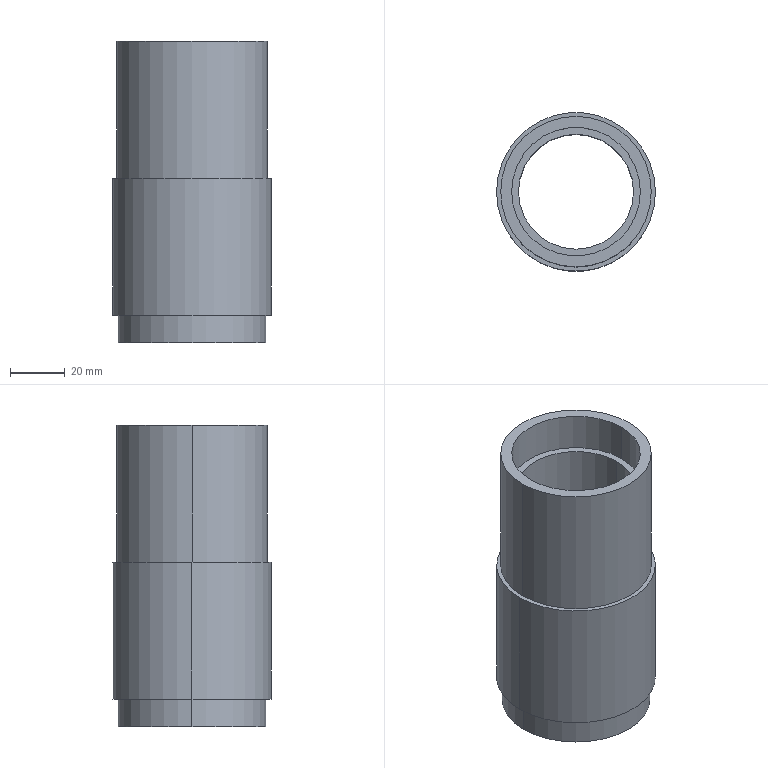Part | SolidWorks | features BaseBody 1 | 1 solid | 18 faces | box 58 x 58 x 110 mm | volume 111613 mm3 | cylinder 12 | plane 6 | commonest cylinder face diameters 47 x4 42 x2 54 x2 55 x2 58 x2
STEP:
#1=CARTESIAN_POINT('',(-27.5,0.,60.));
#2=VERTEX_POINT('',#1);
#3=CARTESIAN_POINT('',(-27.5,0.,110.));
#4=VERTEX_POINT('',#3);
#5=CARTESIAN_POINT('',(-27.5,0.,60.));
#6=DIRECTION('',(0.,0.,1.));
#7=VECTOR('',#6,1000.);
#8=LINE('',#5,#7);
#9=EDGE_CURVE('',#2,#4,#8,.T.);
#10=ORIENTED_EDGE('',*,*,#9,.F.);
#11=CARTESIAN_POINT('',(27.5,0.,60.));
#12=VERTEX_POINT('',#11);
#13=CARTESIAN_POINT('',(0.,0.,60.));
#14=DIRECTION('',(0.,0.,1.));
#15=DIRECTION('',(1.,0.,0.));
#16=AXIS2_PLACEMENT_3D('',#13,#14,#15);
#17=CIRCLE('',#16,27.5);
#18=EDGE_CURVE('',#2,#12,#17,.T.);
#19=ORIENTED_EDGE('',*,*,#18,.T.);
#20=CARTESIAN_POINT('',(27.5,0.,110.));
#21=VERTEX_POINT('',#20);
#22=CARTESIAN_POINT('',(27.5,0.,60.));
#23=DIRECTION('',(0.,0.,1.));
#24=VECTOR('',#23,1000.);
#25=LINE('',#22,#24);
#26=EDGE_CURVE('',#12,#21,#25,.T.);
#27=ORIENTED_EDGE('',*,*,#26,.T.);
#28=CARTESIAN_POINT('',(0.,0.,110.));
#29=DIRECTION('',(0.,0.,1.));
#30=DIRECTION('',(1.,0.,0.));
#31=AXIS2_PLACEMENT_3D('',#28,#29,#30);
#32=CIRCLE('',#31,27.5);
#33=EDGE_CURVE('',#4,#21,#32,.T.);
#34=ORIENTED_EDGE('',*,*,#33,.F.);
#35=EDGE_LOOP('',(#10,#19,#27,#34));
#36=FACE_OUTER_BOUND('',#35,.T.);
#37=CARTESIAN_POINT('',(0.,0.,60.));
#38=DIRECTION('',(0.,0.,1.));
#39=DIRECTION('',(1.,0.,0.));
#40=AXIS2_PLACEMENT_3D('',#37,#38,#39);
#41=CYLINDRICAL_SURFACE('',#40,27.5);
#42=ADVANCED_FACE('',(#36),#41,.T.);
#43=CARTESIAN_POINT('',(0.,0.,60.));
#44=DIRECTION('',(0.,0.,1.));
#45=DIRECTION('',(1.,0.,0.));
#46=AXIS2_PLACEMENT_3D('',#43,#44,#45);
#47=CIRCLE('',#46,27.5);
#48=EDGE_CURVE('',#12,#2,#47,.T.);
#49=ORIENTED_EDGE('',*,*,#48,.F.);
#50=ORIENTED_EDGE('',*,*,#18,.F.);
#51=EDGE_LOOP('',(#49,#50));
#52=FACE_BOUND('',#51,.T.);
#53=CARTESIAN_POINT('',(-29.,0.,60.));
#54=VERTEX_POINT('',#53);
#55=CARTESIAN_POINT('',(29.,0.,60.));
#56=VERTEX_POINT('',#55);
#57=CARTESIAN_POINT('',(0.,0.,60.));
#58=DIRECTION('',(0.,0.,1.));
#59=DIRECTION('',(1.,0.,0.));
#60=AXIS2_PLACEMENT_3D('',#57,#58,#59);
#61=CIRCLE('',#60,29.);
#62=EDGE_CURVE('',#54,#56,#61,.T.);
#63=ORIENTED_EDGE('',*,*,#62,.T.);
#64=CARTESIAN_POINT('',(0.,0.,60.));
#65=DIRECTION('',(0.,0.,1.));
#66=DIRECTION('',(1.,0.,0.));
#67=AXIS2_PLACEMENT_3D('',#64,#65,#66);
#68=CIRCLE('',#67,29.);
#69=EDGE_CURVE('',#56,#54,#68,.T.);
#70=ORIENTED_EDGE('',*,*,#69,.T.);
#71=EDGE_LOOP('',(#63,#70));
#72=FACE_OUTER_BOUND('',#71,.T.);
#73=CARTESIAN_POINT('',(0.,0.,60.));
#74=DIRECTION('',(0.,0.,1.));
#75=DIRECTION('',(1.,0.,0.));
#76=AXIS2_PLACEMENT_3D('',#73,#74,#75);
#77=PLANE('',#76);
#78=ADVANCED_FACE('',(#52,#72),#77,.T.);
#79=CARTESIAN_POINT('',(27.,0.,10.));
#80=VERTEX_POINT('',#79);
#81=CARTESIAN_POINT('',(27.,0.,0.));
#82=VERTEX_POINT('',#81);
#83=CARTESIAN_POINT('',(27.,0.,10.));
#84=DIRECTION('',(0.,0.,-1.));
#85=VECTOR('',#84,1000.);
#86=LINE('',#83,#85);
#87=EDGE_CURVE('',#80,#82,#86,.T.);
#88=ORIENTED_EDGE('',*,*,#87,.F.);
#89=CARTESIAN_POINT('',(-27.,0.,10.));
#90=VERTEX_POINT('',#89);
#91=CARTESIAN_POINT('',(0.,0.,10.));
#92=DIRECTION('',(0.,0.,-1.));
#93=DIRECTION('',(-1.,0.,0.));
#94=AXIS2_PLACEMENT_3D('',#91,#92,#93);
#95=CIRCLE('',#94,27.);
#96=EDGE_CURVE('',#80,#90,#95,.T.);
#97=ORIENTED_EDGE('',*,*,#96,.T.);
#98=CARTESIAN_POINT('',(-27.,0.,0.));
#99=VERTEX_POINT('',#98);
#100=CARTESIAN_POINT('',(-27.,0.,10.));
#101=DIRECTION('',(0.,0.,-1.));
#102=VECTOR('',#101,1000.);
#103=LINE('',#100,#102);
#104=EDGE_CURVE('',#90,#99,#103,.T.);
#105=ORIENTED_EDGE('',*,*,#104,.T.);
#106=CARTESIAN_POINT('',(0.,0.,0.));
#107=DIRECTION('',(0.,0.,-1.));
#108=DIRECTION('',(-1.,0.,0.));
#109=AXIS2_PLACEMENT_3D('',#106,#107,#108);
#110=CIRCLE('',#109,27.);
#111=EDGE_CURVE('',#82,#99,#110,.T.);
#112=ORIENTED_EDGE('',*,*,#111,.F.);
#113=EDGE_LOOP('',(#88,#97,#105,#112));
#114=FACE_OUTER_BOUND('',#113,.T.);
#115=CARTESIAN_POINT('',(0.,0.,10.));
#116=DIRECTION('',(0.,0.,-1.));
#117=DIRECTION('',(-1.,0.,0.));
#118=AXIS2_PLACEMENT_3D('',#115,#116,#117);
#119=CYLINDRICAL_SURFACE('',#118,27.);
#120=ADVANCED_FACE('',(#114),#119,.T.);
#121=CARTESIAN_POINT('',(0.,0.,10.));
#122=DIRECTION('',(0.,0.,-1.));
#123=DIRECTION('',(-1.,0.,0.));
#124=AXIS2_PLACEMENT_3D('',#121,#122,#123);
#125=CIRCLE('',#124,27.);
#126=EDGE_CURVE('',#90,#80,#125,.T.);
#127=ORIENTED_EDGE('',*,*,#126,.F.);
#128=ORIENTED_EDGE('',*,*,#96,.F.);
#129=EDGE_LOOP('',(#127,#128));
#130=FACE_BOUND('',#129,.T.);
#131=CARTESIAN_POINT('',(-29.,0.,10.));
#132=VERTEX_POINT('',#131);
#133=CARTESIAN_POINT('',(29.,0.,10.));
#134=VERTEX_POINT('',#133);
#135=CARTESIAN_POINT('',(0.,0.,10.));
#136=DIRECTION('',(0.,0.,-1.));
#137=DIRECTION('',(-1.,0.,0.));
#138=AXIS2_PLACEMENT_3D('',#135,#136,#137);
#139=CIRCLE('',#138,29.);
#140=EDGE_CURVE('',#132,#134,#139,.T.);
#141=ORIENTED_EDGE('',*,*,#140,.T.);
#142=CARTESIAN_POINT('',(0.,0.,10.));
#143=DIRECTION('',(0.,0.,-1.));
#144=DIRECTION('',(-1.,0.,0.));
#145=AXIS2_PLACEMENT_3D('',#142,#143,#144);
#146=CIRCLE('',#145,29.);
#147=EDGE_CURVE('',#134,#132,#146,.T.);
#148=ORIENTED_EDGE('',*,*,#147,.T.);
#149=EDGE_LOOP('',(#141,#148));
#150=FACE_OUTER_BOUND('',#149,.T.);
#151=CARTESIAN_POINT('',(0.,0.,10.));
#152=DIRECTION('',(0.,0.,-1.));
#153=DIRECTION('',(0.,-1.,0.));
#154=AXIS2_PLACEMENT_3D('',#151,#152,#153);
#155=PLANE('',#154);
#156=ADVANCED_FACE('',(#130,#150),#155,.T.);
#157=CARTESIAN_POINT('',(-23.5,0.,96.));
#158=VERTEX_POINT('',#157);
#159=CARTESIAN_POINT('',(-23.5,0.,110.));
#160=VERTEX_POINT('',#159);
#161=CARTESIAN_POINT('',(-23.5,0.,56.));
#162=DIRECTION('',(0.,0.,1.));
#163=VECTOR('',#162,1000.);
#164=LINE('',#161,#163);
#165=EDGE_CURVE('',#158,#160,#164,.T.);
#166=ORIENTED_EDGE('',*,*,#165,.F.);
#167=CARTESIAN_POINT('',(23.5,0.,96.));
#168=VERTEX_POINT('',#167);
#169=CARTESIAN_POINT('',(0.,0.,96.));
#170=DIRECTION('',(0.,0.,1.));
#171=DIRECTION('',(1.,0.,0.));
#172=AXIS2_PLACEMENT_3D('',#169,#170,#171);
#173=CIRCLE('',#172,23.5);
#174=EDGE_CURVE('',#168,#158,#173,.T.);
#175=ORIENTED_EDGE('',*,*,#174,.F.);
#176=CARTESIAN_POINT('',(23.5,0.,110.));
#177=VERTEX_POINT('',#176);
#178=CARTESIAN_POINT('',(23.5,0.,56.));
#179=DIRECTION('',(0.,0.,1.));
#180=VECTOR('',#179,1000.);
#181=LINE('',#178,#180);
#182=EDGE_CURVE('',#168,#177,#181,.T.);
#183=ORIENTED_EDGE('',*,*,#182,.T.);
#184=CARTESIAN_POINT('',(0.,0.,110.));
#185=DIRECTION('',(0.,0.,1.));
#186=DIRECTION('',(1.,0.,0.));
#187=AXIS2_PLACEMENT_3D('',#184,#185,#186);
#188=CIRCLE('',#187,23.5);
#189=EDGE_CURVE('',#177,#160,#188,.T.);
#190=ORIENTED_EDGE('',*,*,#189,.T.);
#191=EDGE_LOOP('',(#166,#175,#183,#190));
#192=FACE_OUTER_BOUND('',#191,.T.);
#193=CARTESIAN_POINT('',(0.,0.,56.));
#194=DIRECTION('',(0.,0.,1.));
#195=DIRECTION('',(1.,0.,0.));
#196=AXIS2_PLACEMENT_3D('',#193,#194,#195);
#197=CYLINDRICAL_SURFACE('',#196,23.5);
#198=ADVANCED_FACE('',(#192),#197,.F.);
#199=CARTESIAN_POINT('',(21.,0.,96.));
#200=VERTEX_POINT('',#199);
#201=CARTESIAN_POINT('',(-21.,0.,96.));
#202=VERTEX_POINT('',#201);
#203=CARTESIAN_POINT('',(0.,0.,96.));
#204=DIRECTION('',(0.,0.,-1.));
#205=DIRECTION('',(1.,0.,0.));
#206=AXIS2_PLACEMENT_3D('',#203,#204,#205);
#207=CIRCLE('',#206,21.);
#208=EDGE_CURVE('',#200,#202,#207,.T.);
#209=ORIENTED_EDGE('',*,*,#208,.T.);
#210=CARTESIAN_POINT('',(0.,0.,96.));
#211=DIRECTION('',(0.,0.,-1.));
#212=DIRECTION('',(1.,0.,0.));
#213=AXIS2_PLACEMENT_3D('',#210,#211,#212);
#214=CIRCLE('',#213,21.);
#215=EDGE_CURVE('',#202,#200,#214,.T.);
#216=ORIENTED_EDGE('',*,*,#215,.T.);
#217=EDGE_LOOP('',(#209,#216));
#218=FACE_BOUND('',#217,.T.);
#219=ORIENTED_EDGE('',*,*,#174,.T.);
#220=CARTESIAN_POINT('',(0.,0.,96.));
#221=DIRECTION('',(0.,0.,1.));
#222=DIRECTION('',(1.,0.,0.));
#223=AXIS2_PLACEMENT_3D('',#220,#221,#222);
#224=CIRCLE('',#223,23.5);
#225=EDGE_CURVE('',#158,#168,#224,.T.);
#226=ORIENTED_EDGE('',*,*,#225,.T.);
#227=EDGE_LOOP('',(#219,#226));
#228=FACE_OUTER_BOUND('',#227,.T.);
#229=CARTESIAN_POINT('',(0.,0.,96.));
#230=DIRECTION('',(0.,0.,1.));
#231=DIRECTION('',(1.,0.,0.));
#232=AXIS2_PLACEMENT_3D('',#229,#230,#231);
#233=PLANE('',#232);
#234=ADVANCED_FACE('',(#218,#228),#233,.T.);
#235=CARTESIAN_POINT('',(21.,0.,14.));
#236=VERTEX_POINT('',#235);
#237=CARTESIAN_POINT('',(-21.,0.,14.));
#238=VERTEX_POINT('',#237);
#239=CARTESIAN_POINT('',(0.,0.,14.));
#240=DIRECTION('',(0.,0.,-1.));
#241=DIRECTION('',(-1.,0.,0.));
#242=AXIS2_PLACEMENT_3D('',#239,#240,#241);
#243=CIRCLE('',#242,21.);
#244=EDGE_CURVE('',#236,#238,#243,.T.);
#245=ORIENTED_EDGE('',*,*,#244,.F.);
#246=CARTESIAN_POINT('',(0.,0.,14.));
#247=DIRECTION('',(0.,0.,-1.));
#248=DIRECTION('',(-1.,0.,0.));
#249=AXIS2_PLACEMENT_3D('',#246,#247,#248);
#250=CIRCLE('',#249,21.);
#251=EDGE_CURVE('',#238,#236,#250,.T.);
#252=ORIENTED_EDGE('',*,*,#251,.F.);
#253=EDGE_LOOP('',(#245,#252));
#254=FACE_BOUND('',#253,.T.);
#255=CARTESIAN_POINT('',(-23.5,0.,14.));
#256=VERTEX_POINT('',#255);
#257=CARTESIAN_POINT('',(23.5,0.,14.));
#258=VERTEX_POINT('',#257);
#259=CARTESIAN_POINT('',(0.,0.,14.));
#260=DIRECTION('',(0.,0.,-1.));
#261=DIRECTION('',(-1.,0.,0.));
#262=AXIS2_PLACEMENT_3D('',#259,#260,#261);
#263=CIRCLE('',#262,23.5);
#264=EDGE_CURVE('',#256,#258,#263,.T.);
#265=ORIENTED_EDGE('',*,*,#264,.T.);
#266=CARTESIAN_POINT('',(0.,0.,14.));
#267=DIRECTION('',(0.,0.,-1.));
#268=DIRECTION('',(-1.,0.,0.));
#269=AXIS2_PLACEMENT_3D('',#266,#267,#268);
#270=CIRCLE('',#269,23.5);
#271=EDGE_CURVE('',#258,#256,#270,.T.);
#272=ORIENTED_EDGE('',*,*,#271,.T.);
#273=EDGE_LOOP('',(#265,#272));
#274=FACE_OUTER_BOUND('',#273,.T.);
#275=CARTESIAN_POINT('',(0.,0.,14.));
#276=DIRECTION('',(0.,0.,-1.));
#277=DIRECTION('',(0.,-1.,0.));
#278=AXIS2_PLACEMENT_3D('',#275,#276,#277);
#279=PLANE('',#278);
#280=ADVANCED_FACE('',(#254,#274),#279,.T.);
#281=CARTESIAN_POINT('',(23.5,0.,0.));
#282=VERTEX_POINT('',#281);
#283=CARTESIAN_POINT('',(23.5,0.,14.));
#284=DIRECTION('',(0.,0.,-1.));
#285=VECTOR('',#284,1000.);
#286=LINE('',#283,#285);
#287=EDGE_CURVE('',#258,#282,#286,.T.);
#288=ORIENTED_EDGE('',*,*,#287,.F.);
#289=ORIENTED_EDGE('',*,*,#264,.F.);
#290=CARTESIAN_POINT('',(-23.5,0.,0.));
#291=VERTEX_POINT('',#290);
#292=CARTESIAN_POINT('',(-23.5,0.,14.));
#293=DIRECTION('',(0.,0.,-1.));
#294=VECTOR('',#293,1000.);
#295=LINE('',#292,#294);
#296=EDGE_CURVE('',#256,#291,#295,.T.);
#297=ORIENTED_EDGE('',*,*,#296,.T.);
#298=CARTESIAN_POINT('',(0.,0.,0.));
#299=DIRECTION('',(0.,0.,-1.));
#300=DIRECTION('',(-1.,0.,0.));
#301=AXIS2_PLACEMENT_3D('',#298,#299,#300);
#302=CIRCLE('',#301,23.5);
#303=EDGE_CURVE('',#291,#282,#302,.T.);
#304=ORIENTED_EDGE('',*,*,#303,.T.);
#305=EDGE_LOOP('',(#288,#289,#297,#304));
#306=FACE_OUTER_BOUND('',#305,.T.);
#307=CARTESIAN_POINT('',(0.,0.,14.));
#308=DIRECTION('',(0.,0.,-1.));
#309=DIRECTION('',(-1.,0.,0.));
#310=AXIS2_PLACEMENT_3D('',#307,#308,#309);
#311=CYLINDRICAL_SURFACE('',#310,23.5);
#312=ADVANCED_FACE('',(#306),#311,.F.);
#313=CARTESIAN_POINT('',(-21.,0.,58.));
#314=DIRECTION('',(0.,0.,1.));
#315=VECTOR('',#314,1000.);
#316=LINE('',#313,#315);
#317=EDGE_CURVE('',#238,#202,#316,.T.);
#318=ORIENTED_EDGE('',*,*,#317,.F.);
#319=ORIENTED_EDGE('',*,*,#251,.T.);
#320=CARTESIAN_POINT('',(21.,0.,58.));
#321=DIRECTION('',(0.,0.,1.));
#322=VECTOR('',#321,1000.);
#323=LINE('',#320,#322);
#324=EDGE_CURVE('',#236,#200,#323,.T.);
#325=ORIENTED_EDGE('',*,*,#324,.T.);
#326=ORIENTED_EDGE('',*,*,#215,.F.);
#327=EDGE_LOOP('',(#318,#319,#325,#326));
#328=FACE_OUTER_BOUND('',#327,.T.);
#329=CARTESIAN_POINT('',(0.,0.,58.));
#330=DIRECTION('',(0.,0.,1.));
#331=DIRECTION('',(1.,0.,0.));
#332=AXIS2_PLACEMENT_3D('',#329,#330,#331);
#333=CYLINDRICAL_SURFACE('',#332,21.);
#334=ADVANCED_FACE('',(#328),#333,.F.);
#335=ORIENTED_EDGE('',*,*,#303,.F.);
#336=CARTESIAN_POINT('',(0.,0.,0.));
#337=DIRECTION('',(0.,0.,-1.));
#338=DIRECTION('',(-1.,0.,0.));
#339=AXIS2_PLACEMENT_3D('',#336,#337,#338);
#340=CIRCLE('',#339,23.5);
#341=EDGE_CURVE('',#282,#291,#340,.T.);
#342=ORIENTED_EDGE('',*,*,#341,.F.);
#343=EDGE_LOOP('',(#335,#342));
#344=FACE_BOUND('',#343,.T.);
#345=CARTESIAN_POINT('',(0.,0.,0.));
#346=DIRECTION('',(0.,0.,-1.));
#347=DIRECTION('',(-1.,0.,0.));
#348=AXIS2_PLACEMENT_3D('',#345,#346,#347);
#349=CIRCLE('',#348,27.);
#350=EDGE_CURVE('',#99,#82,#349,.T.);
#351=ORIENTED_EDGE('',*,*,#350,.T.);
#352=ORIENTED_EDGE('',*,*,#111,.T.);
#353=EDGE_LOOP('',(#351,#352));
#354=FACE_OUTER_BOUND('',#353,.T.);
#355=CARTESIAN_POINT('',(0.,0.,0.));
#356=DIRECTION('',(0.,0.,1.));
#357=DIRECTION('',(1.,0.,0.));
#358=AXIS2_PLACEMENT_3D('',#355,#356,#357);
#359=PLANE('',#358);
#360=ADVANCED_FACE('',(#344,#354),#359,.F.);
#361=ORIENTED_EDGE('',*,*,#189,.F.);
#362=CARTESIAN_POINT('',(0.,0.,110.));
#363=DIRECTION('',(0.,0.,1.));
#364=DIRECTION('',(1.,0.,0.));
#365=AXIS2_PLACEMENT_3D('',#362,#363,#364);
#366=CIRCLE('',#365,23.5);
#367=EDGE_CURVE('',#160,#177,#366,.T.);
#368=ORIENTED_EDGE('',*,*,#367,.F.);
#369=EDGE_LOOP('',(#361,#368));
#370=FACE_BOUND('',#369,.T.);
#371=CARTESIAN_POINT('',(0.,0.,110.));
#372=DIRECTION('',(0.,0.,1.));
#373=DIRECTION('',(1.,0.,0.));
#374=AXIS2_PLACEMENT_3D('',#371,#372,#373);
#375=CIRCLE('',#374,27.5);
#376=EDGE_CURVE('',#21,#4,#375,.T.);
#377=ORIENTED_EDGE('',*,*,#376,.T.);
#378=ORIENTED_EDGE('',*,*,#33,.T.);
#379=EDGE_LOOP('',(#377,#378));
#380=FACE_OUTER_BOUND('',#379,.T.);
#381=CARTESIAN_POINT('',(0.,0.,110.));
#382=DIRECTION('',(0.,0.,1.));
#383=DIRECTION('',(1.,0.,0.));
#384=AXIS2_PLACEMENT_3D('',#381,#382,#383);
#385=PLANE('',#384);
#386=ADVANCED_FACE('',(#370,#380),#385,.T.);
#387=CARTESIAN_POINT('',(29.,0.,70.));
#388=DIRECTION('',(0.,0.,-1.));
#389=VECTOR('',#388,1000.);
#390=LINE('',#387,#389);
#391=EDGE_CURVE('',#56,#134,#390,.T.);
#392=ORIENTED_EDGE('',*,*,#391,.F.);
#393=ORIENTED_EDGE('',*,*,#62,.F.);
#394=CARTESIAN_POINT('',(-29.,0.,70.));
#395=DIRECTION('',(0.,0.,-1.));
#396=VECTOR('',#395,1000.);
#397=LINE('',#394,#396);
#398=EDGE_CURVE('',#54,#132,#397,.T.);
#399=ORIENTED_EDGE('',*,*,#398,.T.);
#400=ORIENTED_EDGE('',*,*,#147,.F.);
#401=EDGE_LOOP('',(#392,#393,#399,#400));
#402=FACE_OUTER_BOUND('',#401,.T.);
#403=CARTESIAN_POINT('',(0.,0.,70.));
#404=DIRECTION('',(0.,0.,-1.));
#405=DIRECTION('',(-1.,0.,0.));
#406=AXIS2_PLACEMENT_3D('',#403,#404,#405);
#407=CYLINDRICAL_SURFACE('',#406,29.);
#408=ADVANCED_FACE('',(#402),#407,.T.);
#409=ORIENTED_EDGE('',*,*,#69,.F.);
#410=ORIENTED_EDGE('',*,*,#391,.T.);
#411=ORIENTED_EDGE('',*,*,#140,.F.);
#412=ORIENTED_EDGE('',*,*,#398,.F.);
#413=EDGE_LOOP('',(#409,#410,#411,#412));
#414=FACE_OUTER_BOUND('',#413,.T.);
#415=CARTESIAN_POINT('',(0.,0.,70.));
#416=DIRECTION('',(0.,0.,-1.));
#417=DIRECTION('',(-1.,0.,0.));
#418=AXIS2_PLACEMENT_3D('',#415,#416,#417);
#419=CYLINDRICAL_SURFACE('',#418,29.);
#420=ADVANCED_FACE('',(#414),#419,.T.);
#421=ORIENTED_EDGE('',*,*,#244,.T.);
#422=ORIENTED_EDGE('',*,*,#317,.T.);
#423=ORIENTED_EDGE('',*,*,#208,.F.);
#424=ORIENTED_EDGE('',*,*,#324,.F.);
#425=EDGE_LOOP('',(#421,#422,#423,#424));
#426=FACE_OUTER_BOUND('',#425,.T.);
#427=CARTESIAN_POINT('',(0.,0.,58.));
#428=DIRECTION('',(0.,0.,1.));
#429=DIRECTION('',(1.,0.,0.));
#430=AXIS2_PLACEMENT_3D('',#427,#428,#429);
#431=CYLINDRICAL_SURFACE('',#430,21.);
#432=ADVANCED_FACE('',(#426),#431,.F.);
#433=ORIENTED_EDGE('',*,*,#271,.F.);
#434=ORIENTED_EDGE('',*,*,#287,.T.);
#435=ORIENTED_EDGE('',*,*,#341,.T.);
#436=ORIENTED_EDGE('',*,*,#296,.F.);
#437=EDGE_LOOP('',(#433,#434,#435,#436));
#438=FACE_OUTER_BOUND('',#437,.T.);
#439=CARTESIAN_POINT('',(0.,0.,14.));
#440=DIRECTION('',(0.,0.,-1.));
#441=DIRECTION('',(-1.,0.,0.));
#442=AXIS2_PLACEMENT_3D('',#439,#440,#441);
#443=CYLINDRICAL_SURFACE('',#442,23.5);
#444=ADVANCED_FACE('',(#438),#443,.F.);
#445=ORIENTED_EDGE('',*,*,#225,.F.);
#446=ORIENTED_EDGE('',*,*,#165,.T.);
#447=ORIENTED_EDGE('',*,*,#367,.T.);
#448=ORIENTED_EDGE('',*,*,#182,.F.);
#449=EDGE_LOOP('',(#445,#446,#447,#448));
#450=FACE_OUTER_BOUND('',#449,.T.);
#451=CARTESIAN_POINT('',(0.,0.,56.));
#452=DIRECTION('',(0.,0.,1.));
#453=DIRECTION('',(1.,0.,0.));
#454=AXIS2_PLACEMENT_3D('',#451,#452,#453);
#455=CYLINDRICAL_SURFACE('',#454,23.5);
#456=ADVANCED_FACE('',(#450),#455,.F.);
#457=ORIENTED_EDGE('',*,*,#126,.T.);
#458=ORIENTED_EDGE('',*,*,#87,.T.);
#459=ORIENTED_EDGE('',*,*,#350,.F.);
#460=ORIENTED_EDGE('',*,*,#104,.F.);
#461=EDGE_LOOP('',(#457,#458,#459,#460));
#462=FACE_OUTER_BOUND('',#461,.T.);
#463=CARTESIAN_POINT('',(0.,0.,10.));
#464=DIRECTION('',(0.,0.,-1.));
#465=DIRECTION('',(-1.,0.,0.));
#466=AXIS2_PLACEMENT_3D('',#463,#464,#465);
#467=CYLINDRICAL_SURFACE('',#466,27.);
#468=ADVANCED_FACE('',(#462),#467,.T.);
#469=ORIENTED_EDGE('',*,*,#48,.T.);
#470=ORIENTED_EDGE('',*,*,#9,.T.);
#471=ORIENTED_EDGE('',*,*,#376,.F.);
#472=ORIENTED_EDGE('',*,*,#26,.F.);
#473=EDGE_LOOP('',(#469,#470,#471,#472));
#474=FACE_OUTER_BOUND('',#473,.T.);
#475=CARTESIAN_POINT('',(0.,0.,60.));
#476=DIRECTION('',(0.,0.,1.));
#477=DIRECTION('',(1.,0.,0.));
#478=AXIS2_PLACEMENT_3D('',#475,#476,#477);
#479=CYLINDRICAL_SURFACE('',#478,27.5);
#480=ADVANCED_FACE('',(#474),#479,.T.);
#481=CLOSED_SHELL('',(#42,#78,#120,#156,#198,#234,#280,#312,#334,#360,#386,#408,#420,#432,#444,#456,#468,#480));
#482=MANIFOLD_SOLID_BREP('',#481);
#483=CARTESIAN_POINT('',(0.,0.,0.));
#484=DIRECTION('',(0.,0.,1.));
#485=DIRECTION('',(1.,0.,0.));
#486=AXIS2_PLACEMENT_3D('',#483,#484,#485);
#487=(LENGTH_UNIT()NAMED_UNIT(*)SI_UNIT(.MILLI.,.METRE.));
#488=UNCERTAINTY_MEASURE_WITH_UNIT(LENGTH_MEASURE(0.00001),#487,'','');
#489=(NAMED_UNIT(*)PLANE_ANGLE_UNIT()SI_UNIT($,.RADIAN.));
#490=(NAMED_UNIT(*)SI_UNIT($,.STERADIAN.)SOLID_ANGLE_UNIT());
#491=(GEOMETRIC_REPRESENTATION_CONTEXT(3)GLOBAL_UNCERTAINTY_ASSIGNED_CONTEXT((#488))GLOBAL_UNIT_ASSIGNED_CONTEXT((#487,#489,#490))REPRESENTATION_CONTEXT('',''));
#492=ADVANCED_BREP_SHAPE_REPRESENTATION('',(#482,#486),#491);